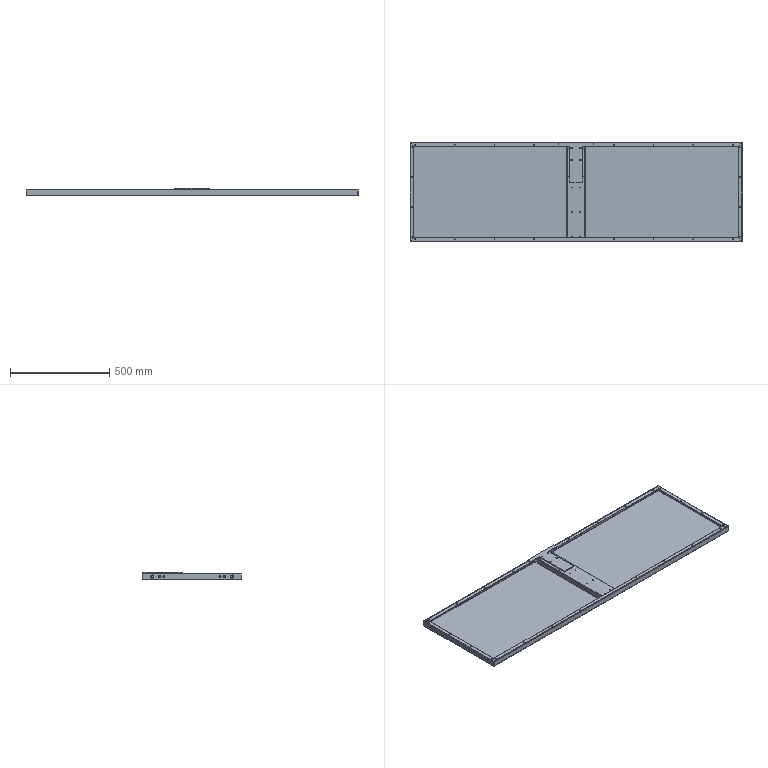Part | NX | features BREP 7 | 40 solids | 1128 faces | box 1670 x 500 x 36 mm | volume 1288518 mm3 | cone 552 | plane 352 | cylinder 208 | spline 16 | commonest cylinder face diameters 4 x48 4.5 x48 3.3 x20 6.8 x20 6 x16 6.6 x16